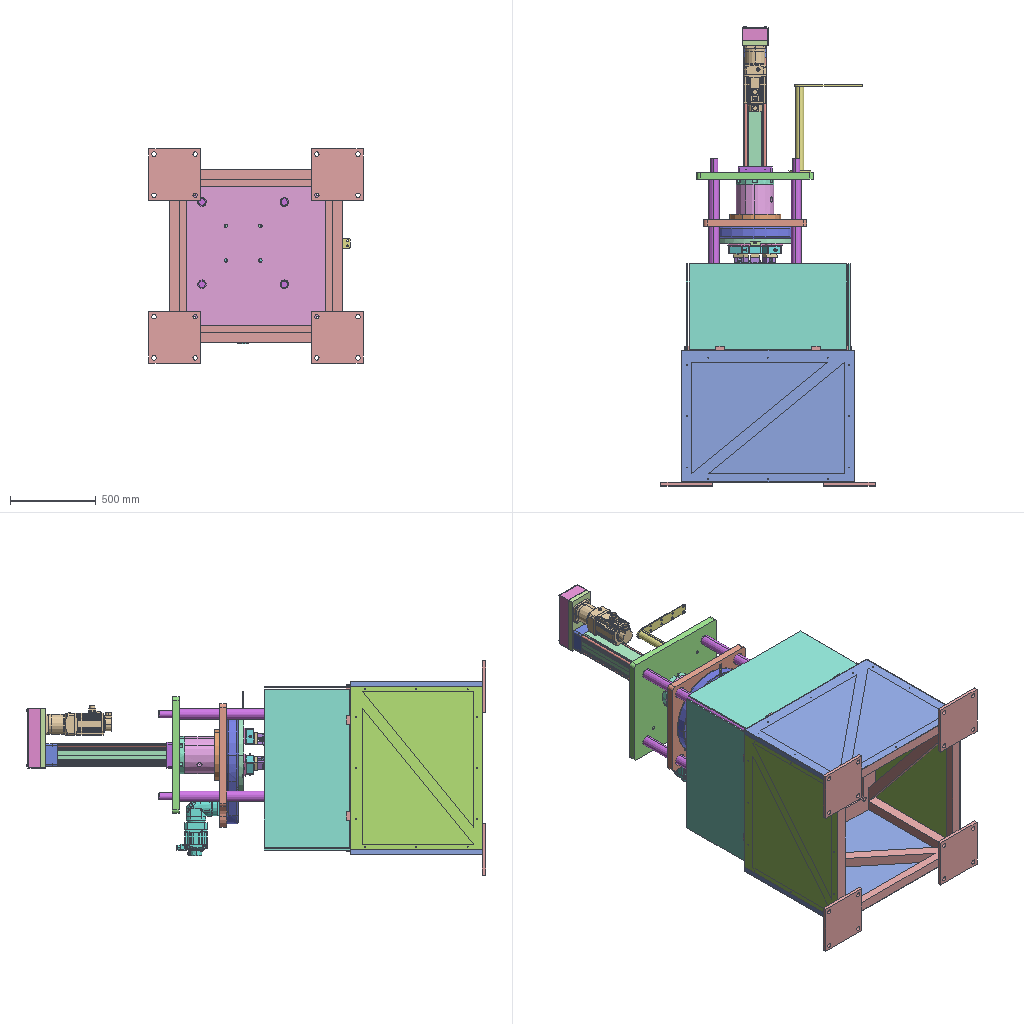Assembly | SolidWorks | 41 different items | 88 placed | box 1250 x 2684 x 1250 mm
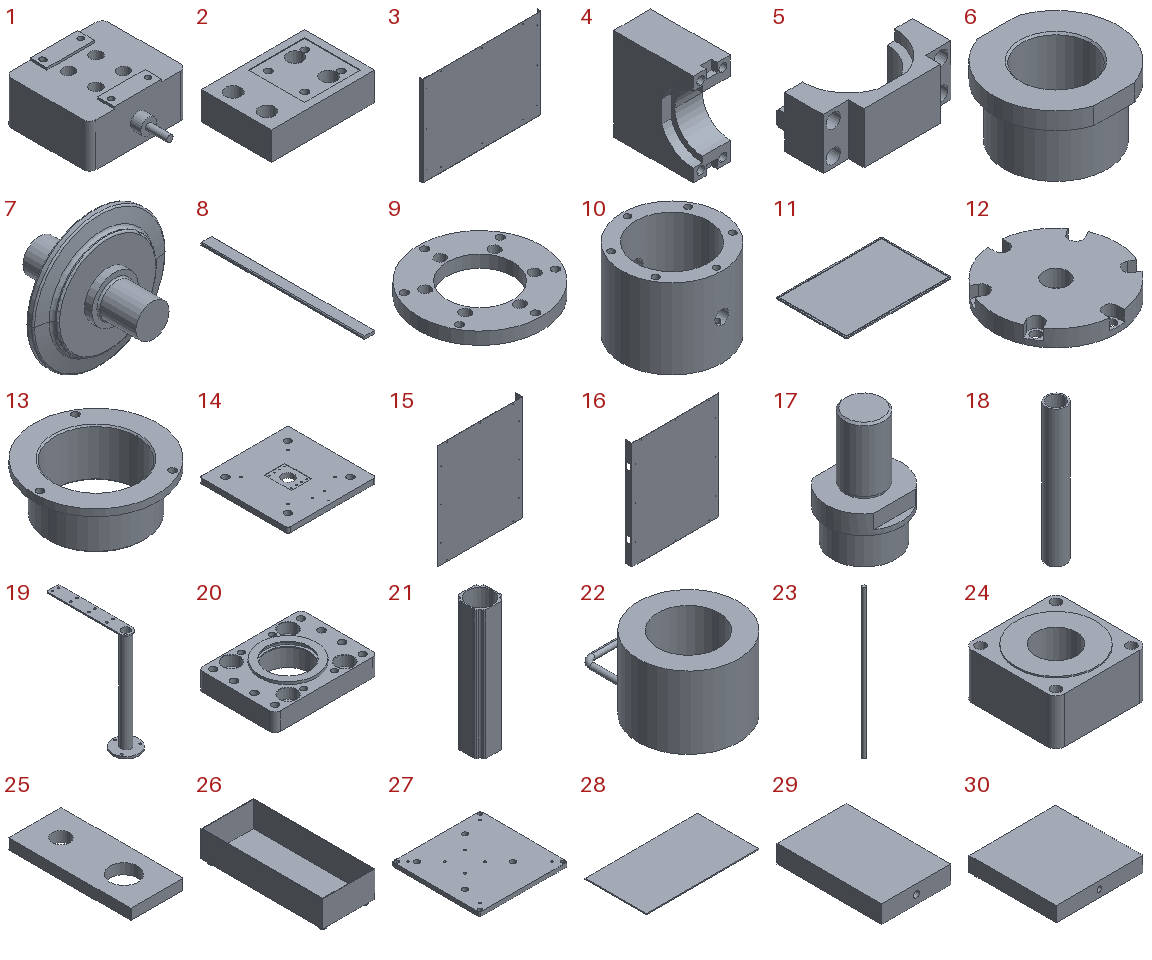Parts list (item | quantity | size | volume | features):
1 | x3 | 92 x 110 x 45 mm | 294451 mm3 | features ICE 6, Extrusion 1, Fillet 1, HoleWzd 1
2 | x3 | 74 x 50 x 23 mm | 67319 mm3 | features ICE 4, Chamfer 1, Extrusion 1
3 | x2 | 1013 x 60 x 770 mm | 1313614 mm3 | features ICE 5, Fillet 3, Extrusion 1, Rip 1
4 | x6 | 20 x 43 x 50 mm | 32312 mm3 | features ICE 4, HoleWzd 2, Extrusion 1
5 | x6 | 50 x 24 x 20 mm | 9639 mm3 | features ICE 5, Chamfer 1, Extrusion 1
6 | x6 | 36 x 34 x 20 mm | 9314 mm3 | features Chamfer 1, Extrusion 1, ICE 1
7 | x3 | 80 x 68 x 80 mm | 71844 mm3 | features Revolution 1
8 | x1 | 15 x 220 x 4 mm | 12760 mm3 | features Chamfer 1, Extrusion 1
9 | x1 | 300 x 300 x 30 mm | 1392605 mm3 | features ICE 3, Extrusion 1
10 | x1 | 220 x 220 x 175 mm | 2942854 mm3 | features Extrusion 1, ICE 1
11 | x1 | 180 x 120 x 2 mm | 42903 mm3 | features Extrusion 1, ICE 1
12 | x1 | 220 x 220 x 30 mm | 1009459 mm3 | features Extrusion 1, ICE 1
13 | x4 | 90 x 90 x 35 mm | 47708 mm3 | features ICE 2, Chamfer 1, Extrusion 1
14 | x1 | 680 x 680 x 40 mm | 17772627 mm3 | features ICE 6, Extrusion 1, Fillet 1
15 | x2 | 770 x 60 x 950 mm | 1175242 mm3 | features ICE 3, Extrusion 1
16 | x1 | 770 x 60 x 950 mm | 1175242 mm3 | features ICE 3, Extrusion 1
17 | x1 | 79 x 79 x 123 mm | 304126 mm3 | features ICE 4, Chamfer 1, Extrusion 1
18 | x1 | 80 x 80 x 550 mm | 2447293 mm3 | features Extrusion 1, ICE 1
19 | x1 | 130 x 430 x 510 mm | 596255 mm3 | features ICE 4, Extrusion 1, Fillet 1
20 | x1 | 200 x 150 x 45 mm | 772010 mm3 | features ICE 9, Chamfer 1, Extrusion 1
21 | x1 | 134 x 134 x 640 mm | 2400423 mm3 | features Extrusion 1
22 | x2 | 180 x 225.589 x 130 mm | 2375464 mm3 | features Extrusion 1, ICE 1, Sweep 1
23 | x4 | 16 x 16 x 669 mm | 134510 mm3 | features Extrusion 1
24 | x1 | 134 x 134 x 71 mm | 961535 mm3 | features ICE 5, HoleWzd 3, Extrusion 1, Fillet 1
25 | x1 | 150 x 350 x 30 mm | 1365196 mm3 | features Extrusion 1, Fillet 1, ICE 1
26 | x1 | 150 x 350 x 85 mm | 254199 mm3 | features Extrusion 1, ICE 1, Shell 1
27 | x1 | 880 x 880 x 40 mm | 30404621 mm3 | features Extrusion 1, ICE 1
28 | x4 | 920 x 500 x 8 mm | 3680000 mm3 | features Extrusion 1
29 | x4 | 116 x 176 x 30 mm | 598351 mm3 | features Extrusion 1, ICE 1
30 | x4 | 176 x 176 x 30 mm | 915151 mm3 | features Extrusion 1, ICE 1
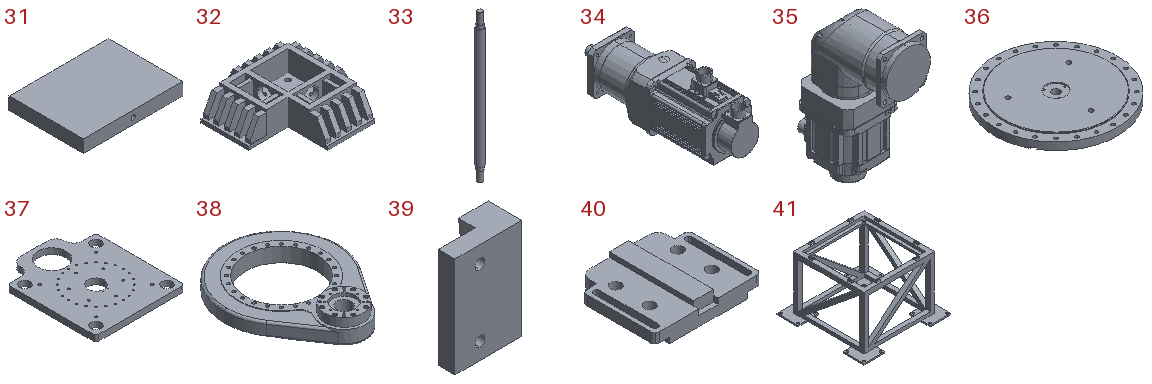31 | x4 | 236 x 176 x 30 mm | 1231951 mm3 | features Extrusion 1, ICE 1
32 | x1 | 857 x 857 x 210 mm | 50598262 mm3 | features ICE 11, Extrusion 1
33 | x4 | 60 x 60 x 1240 mm | 3194362 mm3 | features ICE 4, Chamfer 1, Extrusion 1
34 | x1 | - | - | features BaseBody 1, RefSurface 1
35 | x1 | 130.933 x 261.25 x 349.9 mm | 4855560 mm3 | features BaseBody 2, CombineBodies 1
36 | x1 | 490 x 490 x 35 mm | 5964420 mm3 | features ICE 5, HoleWzd 4, CirPattern 2, Chamfer 1, Extrusion 1, MirrorPattern 1
37 | x1 | 600 x 720 x 40 mm | 13513798 mm3 | features Extrusion 1, HoleWzd 1, ICE 1, LPattern 1
38 | x1 | 540 x 671 x 111 mm | 11365410 mm3 | features ICE 12, CirPattern 2, Chamfer 1, Extrusion 1, Fillet 1, HoleWzd 1, RevCut 1
39 | x1 | 40 x 20 x 60 mm | 32417 mm3 | features ICE 3, Extrusion 1
40 | x3 | 110 x 92 x 21 mm | 133091 mm3 | features ICE 5, Extrusion 1
41 | x1 | 1250 x 1250 x 815 mm | 62783238 mm3 | features ICE 8, CirPattern 3, Extrusion 1, Fillet 1
Mates (type | each side: item.copy, entity, surface, feature):
Coincident | 41.1 face plane Boss-Extrude1 | 3.1 face plane Boss-Extrude1
Width | 3.1 face plane Boss-Extrude1 | 3.1 face plane Boss-Extrude1 | 41.1 face plane Boss-Extrude1 | 41.1 face plane Boss-Extrude1
Coincident | 41.1 face plane Boss-Extrude1 | 3.1 face plane Boss-Extrude2
Coincident | 41.1 face plane Boss-Extrude1 | 15.1 face plane Boss-Extrude1 | 2 times
Width | 3.1 face plane Boss-Extrude1 | 3.2 face plane Boss-Extrude1 | 15.1 face plane Boss-Extrude1 | 15.1 face plane Boss-Extrude1
Coincident | 41.1 face plane Boss-Extrude2 | 27.1 face plane Boss-Extrude1
Width | 15.2 face plane Boss-Extrude1 | 15.1 face plane Boss-Extrude1 | 27.1 face plane Boss-Extrude1 | 27.1 face plane Boss-Extrude1
Width | 3.1 face plane Boss-Extrude1 | 3.2 face plane Boss-Extrude1 | 27.1 face plane Boss-Extrude1 | 27.1 face plane Boss-Extrude1
Width | 41.1 face plane CirPattern4 | 41.1 face plane CirPattern4 | 28.1 face plane Boss-Extrude1 | 28.1 face plane Boss-Extrude1
Coincident | 41.1 face plane CirPattern4 | 28.1 face plane Boss-Extrude1
Width | 3.1 face plane Boss-Extrude1 | 3.2 face plane Boss-Extrude1 | 28.1 face plane Boss-Extrude1 | 28.1 face plane Boss-Extrude1
Coincident | 30.1 face plane Boss-Extrude1 | 31.1 face plane Boss-Extrude1 | 2 times
Coincident | 29.1 face plane Boss-Extrude1 | 31.1 face plane Boss-Extrude1
Coincident | 29.1 face plane Boss-Extrude1 | 30.1 face plane Boss-Extrude1
DistanceDim | 30.1 face plane Boss-Extrude1 | 31.1 face plane Boss-Extrude1
DistanceDim | 29.1 face plane Boss-Extrude1 | 30.1 face plane Boss-Extrude1
Coincident | 27.1 face plane Boss-Extrude1 | 32.1 face plane Boss-Extrude1
Concentric | 27.1 edge | 32.1 edge | 2 times
Coincident | 31.1 face plane Boss-Extrude1 | 32.1 face plane Cut-Extrude3
Coincident | 30.1 face plane Boss-Extrude1 | 32.1 face plane Cut-Extrude3
Width | 32.1 face plane Cut-Extrude3 | 32.1 face plane Cut-Extrude3 | 31.1 face plane Boss-Extrude1 | 31.1 face plane Boss-Extrude1
Coincident | 27.1 face plane Boss-Extrude1 | 11.1 face plane Boss-Extrude1
DistanceDim | 11.1 face plane Boss-Extrude1 | 32.1 face plane Boss-Extrude1
DistanceDim | 32.1 face plane Boss-Extrude1 | 11.1 face plane Boss-Extrude1
Concentric | 32.1 face cylinder Cut-Extrude4 | 22.1 face cylinder Cut-Extrude1
Parallel | 32.1 face plane Boss-Extrude2 | 22.1 plane
Coincident | 32.1 face plane Cut-Extrude3 | 22.1 face plane Boss-Extrude1
Concentric | 32.1 face cylinder Cut-Extrude7 | 22.2 face cylinder Cut-Extrude1
Coincident | 32.1 face plane Cut-Extrude3 | 22.2 face plane Boss-Extrude1
Parallel | 32.1 face plane Boss-Extrude2 | 22.2 plane
Concentric | 27.1 face cylinder Boss-Extrude1 | 33.1 face cylinder Boss-Extrude1
Coincident | 27.1 face plane Boss-Extrude1 | 33.1 face plane Boss-Extrude3
Coincident | 33.2 face plane Boss-Extrude5 | 33.3 face plane Boss-Extrude5
Coincident | 33.2 face plane Boss-Extrude5 | 33.4 face plane Boss-Extrude5
Coincident | 33.1 face plane Boss-Extrude5 | 33.4 face plane Boss-Extrude5
Concentric | 27.1 face cylinder Boss-Extrude1 | 33.4 face cylinder Boss-Extrude3
Concentric | 27.1 face cylinder Boss-Extrude1 | 33.2 face cylinder Boss-Extrude3
Concentric | 27.1 face cylinder Boss-Extrude1 | 33.3 face cylinder Boss-Extrude3
DistanceDim | 37.1 face plane Boss-Extrude1 | 32.1 face plane Boss-Extrude2
Concentric | 33.2 face cylinder Boss-Extrude3 | 37.1 edge
Concentric | 33.3 face cylinder Boss-Extrude3 | 37.1 edge
DistanceDim | 36.1 face plane Boss-Extrude3 | 37.1 face plane Boss-Extrude1
Concentric | 36.1 edge | 37.1 edge
Concentric | 36.1 face cylinder Boss-Extrude2 | 38.1 face cylinder Boss-Extrude1
Concentric | 37.1 face cylinder Boss-Extrude1 | 38.1 face cylinder Boss-Extrude3
Concentric | 36.1 face cylinder Boss-Extrude2 | 39.1 face cylinder Cut-Extrude1
Coincident | 36.1 face plane Boss-Extrude2 | 39.1 face plane Cut-Extrude1
Parallel | 36.1 face plane Cut-Extrude1 | 39.1 face plane Cut-Extrude3
Coincident | 1.1 face plane Boss-Extrude2 | 2.1 face plane Cut-Extrude1
Concentric | 1.1 face cylinder Cut-Extrude2 | 2.1 face cylinder Cut-Extrude2 | 2 times
Coincident | 2.1 face plane Boss-Extrude2 | 4.1 face plane Cut-Extrude4 | 2 times
Coincident | 2.1 face plane Boss-Extrude1 | 4.2 face plane Boss-Extrude1 | 2 times
Coincident | 4.1 face plane Boss-Extrude1 | 4.2 face plane Boss-Extrude1
Coincident | 5.1 face plane Boss-Extrude1 | 4.2 face plane Boss-Extrude1
Concentric | 5.1 face cylinder Cut-Extrude1 | 4.2 face cylinder Cut-Extrude1
Coincident | 5.1 face plane Boss-Extrude2 | 4.2 face plane Cut-Extrude3
Coincident | 4.1 face plane Boss-Extrude1 | 5.2 face plane Boss-Extrude1 | 3 times
Coincident | 2.1 face plane Boss-Extrude1 | 4.1 face plane Boss-Extrude1
Concentric | 4.1 face cylinder Cut-Extrude1 | 7.1 face cylinder Revolve1
Width | 4.2 face plane Boss-Extrude1 | 4.1 face plane Boss-Extrude1 | 7.1 face plane Revolve1 | 7.1 face plane Revolve1
Concentric | 6.1 face cylinder Boss-Extrude1 | 7.1 face cylinder Revolve1
Coincident | 5.1 face plane Cut-Extrude4 | 6.1 face plane Boss-Extrude2
Parallel | 5.1 face plane Boss-Extrude2 | 6.1 face plane Boss-Extrude2
Concentric | 6.1 face cylinder Boss-Extrude1 | 6.2 face cylinder Boss-Extrude1
Coincident | 6.1 face plane Boss-Extrude2 | 6.2 face plane Boss-Extrude2
Coincident | 4.1 face plane Cut-Extrude2 | 6.2 face plane Boss-Extrude2
Coincident | 36.1 face plane Cut-Extrude1 | 40.1 face plane Boss-Extrude2
Parallel | 39.1 face plane Boss-Extrude1 | 40.1 face plane Boss-Extrude1
Width | 40.1 face plane Boss-Extrude2 | 40.1 face plane Boss-Extrude2 | 36.1 face plane Cut-Extrude1 | 36.1 face plane Cut-Extrude1
DistanceDim | 40.1 face plane Boss-Extrude1 | 39.1 face plane Boss-Extrude1
Coincident | 40.1 face plane Cut-Extrude3 | 1.1 face plane Boss-Extrude3 | 3 times
Width | 1.1 face plane Boss-Extrude1 | 1.1 face plane Boss-Extrude1 | 39.1 face plane Boss-Extrude1 | 39.1 face plane Boss-Extrude1
Parallel | 36.1 face plane Cut-Extrude1 | 37.1 face plane Boss-Extrude1
Coincident | 36.1 face plane Cut-Extrude1 | 8.1 face plane Boss-Extrude1
Width | 36.1 face plane Cut-Extrude1 | 36.1 face plane Cut-Extrude1 | 8.1 face plane Boss-Extrude1 | 8.1 face plane Boss-Extrude1
Coincident | 40.1 face plane Boss-Extrude2 | 8.1 face plane Boss-Extrude1
Coincident | 37.1 face plane Boss-Extrude1 | 38.1 face plane Boss-Extrude3
Concentric | 10.1 face cylinder Boss-Extrude1 | 12.1 face cylinder Boss-Extrude1 | 2 times
Concentric | 10.1 face cylinder Boss-Extrude1 | 9.1 face cylinder Boss-Extrude1
Concentric | 12.1 face cylinder Boss-Extrude1 | 9.1 face cylinder Cut-Extrude2
Coincident | 10.1 face plane Boss-Extrude1 | 9.1 face plane Boss-Extrude1
Coincident | 10.1 face plane Boss-Extrude1 | 12.1 face plane Boss-Extrude1
Concentric | 37.1 face cylinder Boss-Extrude1 | 10.1 face cylinder Boss-Extrude1
Concentric | 37.1 face cylinder Boss-Extrude1 | 9.1 face cylinder Cut-Extrude1
Coincident | 37.1 face plane Boss-Extrude1 | 9.1 face plane Boss-Extrude1
Concentric | 33.1 face cylinder Boss-Extrude3 | 13.1 face cylinder Boss-Extrude1
Coincident | 37.1 face plane Boss-Extrude2 | 13.1 face plane Boss-Extrude2
Concentric | 37.1 face cylinder LPattern1 | 13.1 edge
Concentric | 33.3 face cylinder Boss-Extrude3 | 14.1 face cylinder Cut-Extrude6
Concentric | 33.2 face cylinder Boss-Extrude5 | 14.1 face cylinder Cut-Extrude6
DistanceDim | 14.1 face plane Boss-Extrude1 | 37.1 face plane Boss-Extrude1
Concentric | 14.1 face cylinder Cut-Extrude3 | 17.1 face cylinder Boss-Extrude2
DistanceDim | 17.1 face plane Boss-Extrude2 | 14.1 face plane Boss-Extrude1
Parallel | 14.1 face plane Boss-Extrude1 | 17.1 face plane Cut-Extrude1
Concentric | 17.1 face cylinder Boss-Extrude1 | 18.1 face cylinder Boss-Extrude1
Coincident | 17.1 face plane Boss-Extrude2 | 18.1 face plane Boss-Extrude1
Coincident | 14.1 face plane Boss-Extrude1 | 19.1 face plane Boss-Extrude1
Concentric | 14.1 edge | 19.1 edge | 2 times
Concentric | 18.1 face cylinder Boss-Extrude1 | 20.1 face cylinder Cut-Extrude7
Parallel | 14.1 face plane Boss-Extrude1 | 20.1 face plane Boss-Extrude1
DistanceDim | 20.1 face plane Boss-Extrude1 | 14.1 face plane Boss-Extrude1
Concentric | 18.1 face cylinder Boss-Extrude1 | 21.1 face cylinder Boss-Extrude1
DistanceDim | 37.1 face plane Boss-Extrude1 | 21.1 face plane Boss-Extrude1
Parallel | 20.1 face plane Boss-Extrude1 | 21.1 face plane Boss-Extrude1
Concentric | 20.1 face cylinder Boss-Extrude1 | 23.1 face cylinder Boss-Extrude1
Concentric | 21.1 face cylinder Boss-Extrude1 | 24.1 face cylinder Cut-Extrude1
Concentric | 23.2 face cylinder Boss-Extrude1 | 24.1 face cylinder Cut-Extrude3
Coincident | 23.2 face plane Boss-Extrude1 | 24.1 face plane Boss-Extrude1
Concentric | 24.1 face cylinder Cut-Extrude1 | 25.1 face cylinder Cut-Extrude1
Coincident | 24.1 face plane Boss-Extrude1 | 25.1 face plane Boss-Extrude1
Parallel | 21.1 face plane Boss-Extrude1 | 25.1 face plane Boss-Extrude1
Coincident | 21.1 face plane Boss-Extrude1 | 24.1 face plane Boss-Extrude1
Coincident | 25.1 face plane Boss-Extrude1 | 26.1 face plane Boss-Extrude1 | 3 times
Concentric | 25.1 face cylinder Cut-Extrude1 | 34.1 face cylinder Input1
Coincident | 25.1 face plane Boss-Extrude1 | 34.1 face plane Input1
Parallel | 25.1 face plane Boss-Extrude1 | 34.1 face plane Input1
Concentric | 38.1 face cylinder Cut-Extrude1 | 35.1 face cylinder Input1
Coincident | 38.1 face plane Boss-Extrude3 | 35.1 face plane Input1
Concentric | 38.1 face cylinder CirPattern1 | 35.1 face cylinder Input1
Parallel | 41.1 face plane CirPattern3 | assembly plane
Parallel | 41.1 edge | assembly plane